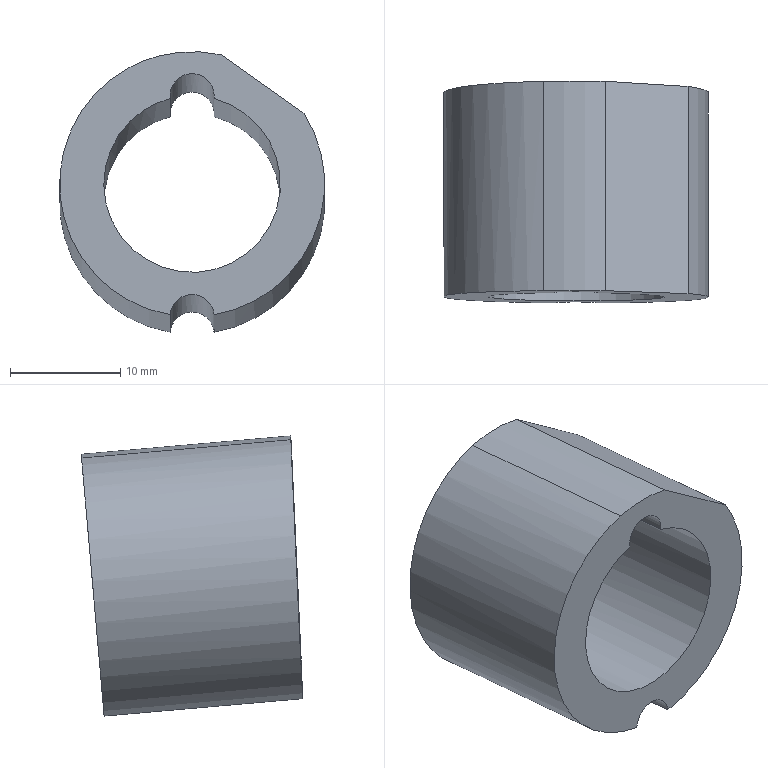Part | NX | features solid 2 | 1 solid | 9 faces | box 24 x 20.067 x 25.402 mm | volume 4320 mm3 | cylinder 5 | plane 3 | spline 1 | commonest cylinder face diameters 4 x2 24 x2 16 x1
STEP:
#1=CARTESIAN_POINT('',(166.66,-27.812,-44.59));
#2=VERTEX_POINT('',#1);
#3=CARTESIAN_POINT('',(158.517,-29.404,-62.778));
#4=VERTEX_POINT('',#3);
#5=CARTESIAN_POINT('',(156.524,-28.372,-50.99));
#6=DIRECTION('',(0.,0.9962,-0.08716));
#7=DIRECTION('',(0.,0.08716,0.9962));
#8=AXIS2_PLACEMENT_3D('',#5,#6,#7);
#9=CIRCLE('',#8,12.);
#10=EDGE_CURVE('',#2,#4,#9,.T.);
#11=ORIENTED_EDGE('',*,*,#10,.F.);
#12=CARTESIAN_POINT('',(166.66,-46.578,-42.949));
#13=VERTEX_POINT('',#12);
#14=CARTESIAN_POINT('',(166.66,-27.812,-44.59));
#15=DIRECTION('',(0.,-0.9962,0.08716));
#16=VECTOR('',#15,1000.);
#17=LINE('',#14,#16);
#18=EDGE_CURVE('',#2,#13,#17,.T.);
#19=ORIENTED_EDGE('',*,*,#18,.T.);
#20=CARTESIAN_POINT('',(158.517,-47.393,-61.204));
#21=VERTEX_POINT('',#20);
#22=CARTESIAN_POINT('',(156.524,-46.851,-49.373));
#23=DIRECTION('',(0.001957,0.999,-0.04546));
#24=DIRECTION('',(0.04675,0.04532,0.9979));
#25=AXIS2_PLACEMENT_3D('',#22,#23,#24);
#26=ELLIPSE('',#25,12.011,12.);
#27=EDGE_CURVE('',#13,#21,#26,.T.);
#28=ORIENTED_EDGE('',*,*,#27,.T.);
#29=CARTESIAN_POINT('',(158.517,-38.489,-61.983));
#30=DIRECTION('',(0.,0.9962,-0.08716));
#31=VECTOR('',#30,1000.);
#32=LINE('',#29,#31);
#33=EDGE_CURVE('',#21,#4,#32,.T.);
#34=ORIENTED_EDGE('',*,*,#33,.T.);
#35=EDGE_LOOP('',(#11,#19,#28,#34));
#36=FACE_BOUND('',#35,.T.);
#37=CARTESIAN_POINT('',(156.524,-28.372,-50.99));
#38=DIRECTION('',(0.,-0.9962,0.08716));
#39=DIRECTION('',(0.,-0.08716,-0.9962));
#40=AXIS2_PLACEMENT_3D('',#37,#38,#39);
#41=CYLINDRICAL_SURFACE('',#40,12.);
#42=ADVANCED_FACE('',(#36),#41,.T.);
#43=CARTESIAN_POINT('',(158.508,-46.502,-41.624));
#44=VERTEX_POINT('',#43);
#45=CARTESIAN_POINT('',(154.539,-46.494,-41.625));
#46=VERTEX_POINT('',#45);
#47=CARTESIAN_POINT('',(156.524,-46.851,-49.373));
#48=DIRECTION('',(0.001957,0.999,-0.04546));
#49=DIRECTION('',(0.04675,0.04532,0.9979));
#50=AXIS2_PLACEMENT_3D('',#47,#48,#49);
#51=ELLIPSE('',#50,8.007,8.);
#52=EDGE_CURVE('',#44,#46,#51,.T.);
#53=ORIENTED_EDGE('',*,*,#52,.F.);
#54=CARTESIAN_POINT('',(158.508,-27.697,-43.269));
#55=VERTEX_POINT('',#54);
#56=CARTESIAN_POINT('',(158.508,-27.697,-43.269));
#57=DIRECTION('',(0.,-0.9962,0.08716));
#58=VECTOR('',#57,1000.);
#59=LINE('',#56,#58);
#60=EDGE_CURVE('',#55,#44,#59,.T.);
#61=ORIENTED_EDGE('',*,*,#60,.F.);
#62=CARTESIAN_POINT('',(154.539,-27.697,-43.269));
#63=VERTEX_POINT('',#62);
#64=CARTESIAN_POINT('',(156.524,-28.372,-50.99));
#65=DIRECTION('',(0.,-0.9962,0.08716));
#66=DIRECTION('',(0.,-0.08716,-0.9962));
#67=AXIS2_PLACEMENT_3D('',#64,#65,#66);
#68=CIRCLE('',#67,8.);
#69=EDGE_CURVE('',#55,#63,#68,.F.);
#70=ORIENTED_EDGE('',*,*,#69,.T.);
#71=CARTESIAN_POINT('',(154.539,-27.697,-43.269));
#72=DIRECTION('',(0.,-0.9962,0.08716));
#73=VECTOR('',#72,1000.);
#74=LINE('',#71,#73);
#75=EDGE_CURVE('',#46,#63,#74,.F.);
#76=ORIENTED_EDGE('',*,*,#75,.F.);
#77=EDGE_LOOP('',(#53,#61,#70,#76));
#78=FACE_BOUND('',#77,.T.);
#79=CARTESIAN_POINT('',(156.524,-28.372,-50.99));
#80=DIRECTION('',(0.,-0.9962,0.08716));
#81=DIRECTION('',(0.,-0.08716,-0.9962));
#82=AXIS2_PLACEMENT_3D('',#79,#80,#81);
#83=CYLINDRICAL_SURFACE('',#82,8.);
#84=ADVANCED_FACE('',(#78),#83,.F.);
#85=CARTESIAN_POINT('',(159.152,-27.352,-39.326));
#86=VERTEX_POINT('',#85);
#87=CARTESIAN_POINT('',(155.444,-27.124,-36.725));
#88=DIRECTION('',(-0.8177,0.05017,0.5734));
#89=VECTOR('',#88,1000.);
#90=LINE('',#87,#89);
#91=EDGE_CURVE('',#2,#86,#90,.T.);
#92=ORIENTED_EDGE('',*,*,#91,.F.);
#93=ORIENTED_EDGE('',*,*,#10,.T.);
#94=CARTESIAN_POINT('',(154.531,-29.404,-62.778));
#95=VERTEX_POINT('',#94);
#96=CARTESIAN_POINT('',(156.524,-29.418,-62.944));
#97=DIRECTION('',(0.,-0.9962,0.08716));
#98=DIRECTION('',(0.,0.08716,0.9962));
#99=AXIS2_PLACEMENT_3D('',#96,#97,#98);
#100=CIRCLE('',#99,2.);
#101=EDGE_CURVE('',#4,#95,#100,.T.);
#102=ORIENTED_EDGE('',*,*,#101,.T.);
#103=CARTESIAN_POINT('',(153.547,-27.359,-39.409));
#104=VERTEX_POINT('',#103);
#105=CARTESIAN_POINT('',(156.524,-28.372,-50.99));
#106=DIRECTION('',(0.,0.9962,-0.08716));
#107=DIRECTION('',(0.,0.08716,0.9962));
#108=AXIS2_PLACEMENT_3D('',#105,#106,#107);
#109=CIRCLE('',#108,12.);
#110=EDGE_CURVE('',#95,#104,#109,.T.);
#111=ORIENTED_EDGE('',*,*,#110,.T.);
#112=CARTESIAN_POINT('',(153.547,-27.359,-39.409));
#113=CARTESIAN_POINT('',(155.5,-27.315,-38.911));
#114=CARTESIAN_POINT('',(157.547,-27.315,-38.911));
#115=CARTESIAN_POINT('',(159.5,-27.359,-39.409));
#116=B_SPLINE_CURVE_WITH_KNOTS('',3,(#112,#113,#114,#115),.UNSPECIFIED.,.F.,.F.,(4,4),(0.,1.),.PIECEWISE_BEZIER_KNOTS.);
#117=EDGE_CURVE('',#104,#86,#116,.T.);
#118=ORIENTED_EDGE('',*,*,#117,.T.);
#119=EDGE_LOOP('',(#92,#93,#102,#111,#118));
#120=FACE_BOUND('',#119,.T.);
#121=CARTESIAN_POINT('',(156.524,-27.675,-43.02));
#122=DIRECTION('',(0.,-0.9962,0.08716));
#123=DIRECTION('',(0.,-0.08716,-0.9962));
#124=AXIS2_PLACEMENT_3D('',#121,#122,#123);
#125=CIRCLE('',#124,2.);
#126=EDGE_CURVE('',#55,#63,#125,.T.);
#127=ORIENTED_EDGE('',*,*,#126,.T.);
#128=ORIENTED_EDGE('',*,*,#69,.F.);
#129=EDGE_LOOP('',(#127,#128));
#130=FACE_BOUND('',#129,.T.);
#131=CARTESIAN_POINT('',(153.547,-27.359,-39.409));
#132=DIRECTION('',(0.,0.9962,-0.08716));
#133=DIRECTION('',(0.,0.08716,0.9962));
#134=AXIS2_PLACEMENT_3D('',#131,#132,#133);
#135=PLANE('',#134);
#136=ADVANCED_FACE('',(#120,#130),#135,.T.);
#137=CARTESIAN_POINT('',(159.152,-46.323,-37.666));
#138=VERTEX_POINT('',#137);
#139=CARTESIAN_POINT('',(162.955,-46.452,-40.342));
#140=DIRECTION('',(-0.8175,0.02778,0.5752));
#141=VECTOR('',#140,1000.);
#142=LINE('',#139,#141);
#143=EDGE_CURVE('',#138,#13,#142,.F.);
#144=ORIENTED_EDGE('',*,*,#143,.F.);
#145=CARTESIAN_POINT('',(153.547,-46.316,-37.75));
#146=VERTEX_POINT('',#145);
#147=CARTESIAN_POINT('',(153.547,-46.316,-37.75));
#148=CARTESIAN_POINT('',(155.38,-46.298,-37.281));
#149=CARTESIAN_POINT('',(157.312,-46.301,-37.253));
#150=CARTESIAN_POINT('',(159.152,-46.323,-37.666));
#151=B_SPLINE_CURVE_WITH_KNOTS('',3,(#147,#148,#149,#150),.UNSPECIFIED.,.F.,.F.,(4,4),(0.,0.005664),.UNSPECIFIED.);
#152=EDGE_CURVE('',#146,#138,#151,.T.);
#153=ORIENTED_EDGE('',*,*,#152,.F.);
#154=CARTESIAN_POINT('',(154.531,-47.385,-61.205));
#155=VERTEX_POINT('',#154);
#156=CARTESIAN_POINT('',(156.524,-46.851,-49.373));
#157=DIRECTION('',(0.001957,0.999,-0.04546));
#158=DIRECTION('',(0.04675,0.04532,0.9979));
#159=AXIS2_PLACEMENT_3D('',#156,#157,#158);
#160=ELLIPSE('',#159,12.011,12.);
#161=EDGE_CURVE('',#155,#146,#160,.T.);
#162=ORIENTED_EDGE('',*,*,#161,.F.);
#163=CARTESIAN_POINT('',(156.524,-47.397,-61.371));
#164=DIRECTION('',(0.001957,0.999,-0.04546));
#165=DIRECTION('',(-0.04675,-0.04532,-0.9979));
#166=AXIS2_PLACEMENT_3D('',#163,#164,#165);
#167=ELLIPSE('',#166,2.002,2.);
#168=EDGE_CURVE('',#155,#21,#167,.T.);
#169=ORIENTED_EDGE('',*,*,#168,.T.);
#170=ORIENTED_EDGE('',*,*,#27,.F.);
#171=EDGE_LOOP('',(#144,#153,#162,#169,#170));
#172=FACE_BOUND('',#171,.T.);
#173=CARTESIAN_POINT('',(156.524,-46.487,-41.374));
#174=DIRECTION('',(0.001957,0.999,-0.04546));
#175=DIRECTION('',(-0.04675,-0.04532,-0.9979));
#176=AXIS2_PLACEMENT_3D('',#173,#174,#175);
#177=ELLIPSE('',#176,2.002,2.);
#178=EDGE_CURVE('',#46,#44,#177,.T.);
#179=ORIENTED_EDGE('',*,*,#178,.T.);
#180=ORIENTED_EDGE('',*,*,#52,.T.);
#181=EDGE_LOOP('',(#179,#180));
#182=FACE_BOUND('',#181,.T.);
#183=CARTESIAN_POINT('',(128.811,-48.589,-88.763));
#184=DIRECTION('',(0.001957,0.999,-0.04546));
#185=DIRECTION('',(0.06617,0.04523,0.9968));
#186=AXIS2_PLACEMENT_3D('',#183,#184,#185);
#187=PLANE('',#186);
#188=ADVANCED_FACE('',(#172,#182),#187,.F.);
#189=ORIENTED_EDGE('',*,*,#110,.F.);
#190=CARTESIAN_POINT('',(154.531,-38.489,-61.983));
#191=DIRECTION('',(0.,0.9962,-0.08716));
#192=VECTOR('',#191,1000.);
#193=LINE('',#190,#192);
#194=EDGE_CURVE('',#95,#155,#193,.F.);
#195=ORIENTED_EDGE('',*,*,#194,.T.);
#196=ORIENTED_EDGE('',*,*,#161,.T.);
#197=CARTESIAN_POINT('',(153.547,-27.359,-39.409));
#198=DIRECTION('',(0.,-0.9962,0.08716));
#199=VECTOR('',#198,1000.);
#200=LINE('',#197,#199);
#201=EDGE_CURVE('',#104,#146,#200,.T.);
#202=ORIENTED_EDGE('',*,*,#201,.F.);
#203=EDGE_LOOP('',(#189,#195,#196,#202));
#204=FACE_BOUND('',#203,.T.);
#205=CARTESIAN_POINT('',(156.524,-28.372,-50.99));
#206=DIRECTION('',(0.,-0.9962,0.08716));
#207=DIRECTION('',(0.,-0.08716,-0.9962));
#208=AXIS2_PLACEMENT_3D('',#205,#206,#207);
#209=CYLINDRICAL_SURFACE('',#208,12.);
#210=ADVANCED_FACE('',(#204),#209,.T.);
#211=ORIENTED_EDGE('',*,*,#152,.T.);
#212=CARTESIAN_POINT('',(159.152,-27.352,-39.326));
#213=DIRECTION('',(0.,-0.9962,0.08716));
#214=VECTOR('',#213,1000.);
#215=LINE('',#212,#214);
#216=EDGE_CURVE('',#138,#86,#215,.F.);
#217=ORIENTED_EDGE('',*,*,#216,.T.);
#218=ORIENTED_EDGE('',*,*,#117,.F.);
#219=ORIENTED_EDGE('',*,*,#201,.T.);
#220=EDGE_LOOP('',(#211,#217,#218,#219));
#221=FACE_BOUND('',#220,.T.);
#222=CARTESIAN_POINT('',(153.547,-27.359,-39.409));
#223=CARTESIAN_POINT('',(153.547,-46.453,-37.738));
#224=CARTESIAN_POINT('',(155.384,-27.318,-38.94));
#225=CARTESIAN_POINT('',(155.384,-46.412,-37.27));
#226=CARTESIAN_POINT('',(157.305,-27.316,-38.913));
#227=CARTESIAN_POINT('',(157.305,-46.409,-37.242));
#228=CARTESIAN_POINT('',(159.152,-27.352,-39.326));
#229=CARTESIAN_POINT('',(159.152,-46.446,-37.655));
#230=B_SPLINE_SURFACE_WITH_KNOTS('',3,1,((#222,#223),(#224,#225),(#226,#227),(#228,#229)),.SURF_OF_LINEAR_EXTRUSION.,.F.,.F.,.F.,(4,4),(2,2),(0.,0.9407),(0.,1.),.PIECEWISE_BEZIER_KNOTS.);
#231=ADVANCED_FACE('',(#221),#230,.F.);
#232=ORIENTED_EDGE('',*,*,#168,.F.);
#233=ORIENTED_EDGE('',*,*,#194,.F.);
#234=ORIENTED_EDGE('',*,*,#101,.F.);
#235=ORIENTED_EDGE('',*,*,#33,.F.);
#236=EDGE_LOOP('',(#232,#233,#234,#235));
#237=FACE_BOUND('',#236,.T.);
#238=CARTESIAN_POINT('',(156.524,-49.342,-61.201));
#239=DIRECTION('',(0.,0.9962,-0.08716));
#240=DIRECTION('',(0.,-0.08716,-0.9962));
#241=AXIS2_PLACEMENT_3D('',#238,#239,#240);
#242=CYLINDRICAL_SURFACE('',#241,2.);
#243=ADVANCED_FACE('',(#237),#242,.F.);
#244=ORIENTED_EDGE('',*,*,#75,.T.);
#245=ORIENTED_EDGE('',*,*,#126,.F.);
#246=ORIENTED_EDGE('',*,*,#60,.T.);
#247=ORIENTED_EDGE('',*,*,#178,.F.);
#248=EDGE_LOOP('',(#244,#245,#246,#247));
#249=FACE_BOUND('',#248,.T.);
#250=CARTESIAN_POINT('',(156.524,-47.599,-41.277));
#251=DIRECTION('',(0.,0.9962,-0.08716));
#252=DIRECTION('',(0.,0.08716,0.9962));
#253=AXIS2_PLACEMENT_3D('',#250,#251,#252);
#254=CYLINDRICAL_SURFACE('',#253,2.);
#255=ADVANCED_FACE('',(#249),#254,.F.);
#256=ORIENTED_EDGE('',*,*,#91,.T.);
#257=ORIENTED_EDGE('',*,*,#216,.F.);
#258=ORIENTED_EDGE('',*,*,#143,.T.);
#259=ORIENTED_EDGE('',*,*,#18,.F.);
#260=EDGE_LOOP('',(#256,#257,#258,#259));
#261=FACE_BOUND('',#260,.T.);
#262=CARTESIAN_POINT('',(159.152,53.296,-46.381));
#263=DIRECTION('',(-0.5756,-0.07127,-0.8146));
#264=DIRECTION('',(-0.8167,0.,0.5771));
#265=AXIS2_PLACEMENT_3D('',#262,#263,#264);
#266=PLANE('',#265);
#267=ADVANCED_FACE('',(#261),#266,.F.);
#268=CLOSED_SHELL('',(#42,#84,#136,#188,#210,#231,#243,#255,#267));
#269=MANIFOLD_SOLID_BREP('',#268);
#270=(LENGTH_UNIT()NAMED_UNIT(*)SI_UNIT(.MILLI.,.METRE.));
#271=UNCERTAINTY_MEASURE_WITH_UNIT(LENGTH_MEASURE(0.0508),#270,'','');
#272=(NAMED_UNIT(*)PLANE_ANGLE_UNIT()SI_UNIT($,.RADIAN.));
#273=(NAMED_UNIT(*)SI_UNIT($,.STERADIAN.)SOLID_ANGLE_UNIT());
#274=(GEOMETRIC_REPRESENTATION_CONTEXT(3)GLOBAL_UNCERTAINTY_ASSIGNED_CONTEXT((#271))GLOBAL_UNIT_ASSIGNED_CONTEXT((#270,#272,#273))REPRESENTATION_CONTEXT('',''));
#275=ADVANCED_BREP_SHAPE_REPRESENTATION('',(#269),#274);